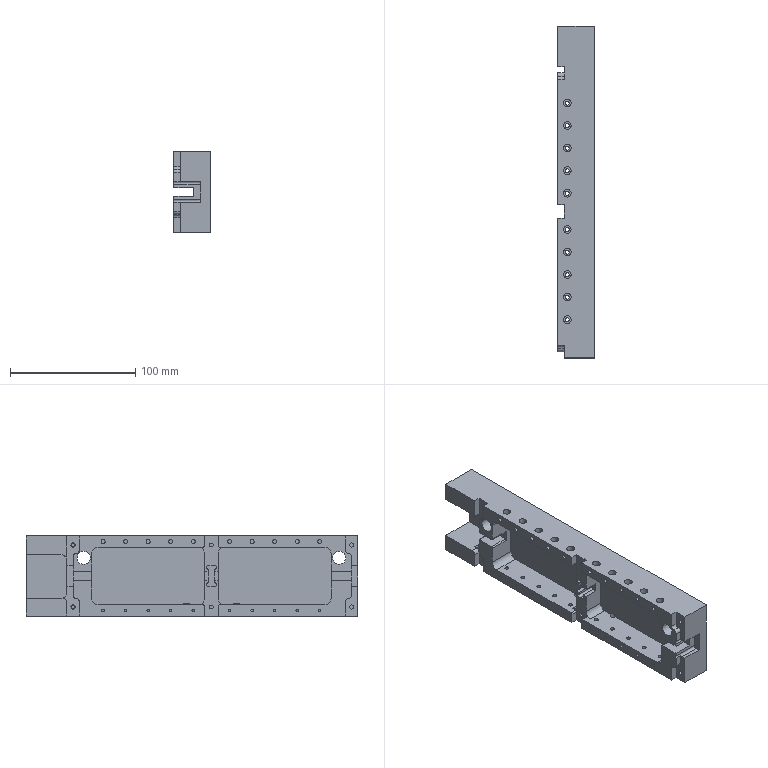Part | 1 solid | 176 faces | box 29 x 265 x 64 mm | volume 262247 mm3 | cylinder 96 | plane 80 | commonest cylinder face diameters 2 x19 3.3 x14 3.1 x10 5 x10 6.1 x10 10 x10